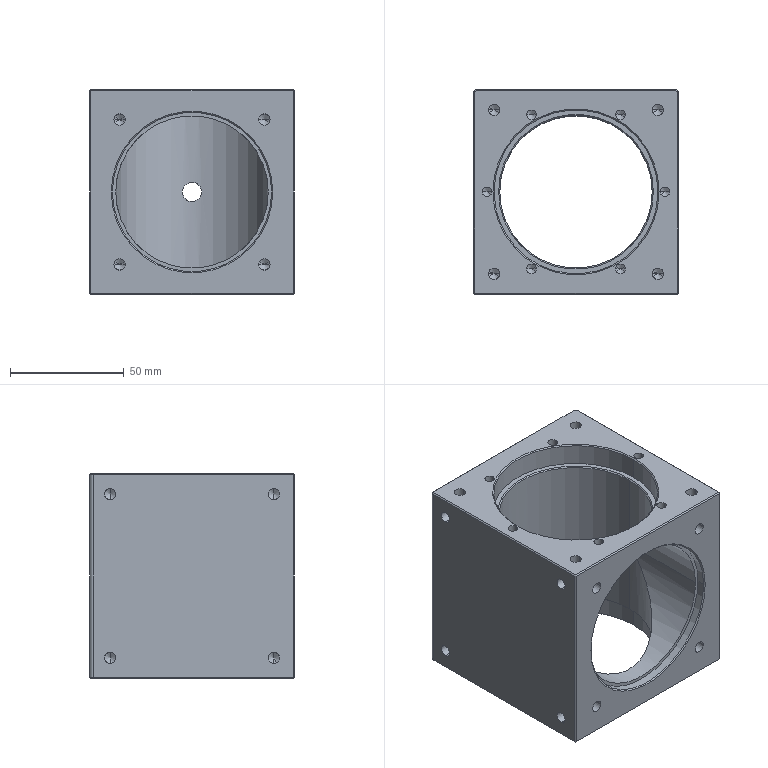NC program | NX | posted with a generic post | part box 90 x 90 x 90 mm
Whole program:
N10 G17 G21 G94 G90
(DRILLING_COPY_1_COPY_1 , TOOL : D6A45)
N12 T07 M6
N14 G54
N16 G17 G0 G90 X-31.82 Y-31.82 B0. C0. S5000 M3
N18 G43 Z30. H7
N20 G94 G81 G98 Z-1. F250. R3.
N22 Y31.82
N24 X0. Y0.
N26 X31.82 Y31.82
N28 Y-31.82
N30 G80
N32 G0 X31.82 Y-31.82 Z30.
N34 M5
(DRILLING_COPY_1_COPY_COPY_COPY_COPY , TOOL : 5.0ZT)
N36 T15 M6
N38 G54
N40 G17 G0 G90 X-31.82 Y-31.82 B0. C0. S2000 M3
N42 G43 Z30. H15
N44 G94 G83 G98 Z-18.502 F150. Q2. R3.
N46 Y31.82
N48 X31.82
N50 Y-31.82
N52 G80
N54 G0 X31.82 Y-31.82 Z30.
N56 M5
(DRILLING_COPY_1_COPY_COPY_COPY_COPY_COPY , TOOL : 9.0ZT)
N58 T09 M6
N60 G54
N62 G17 G0 G90 X0. Y0. B0. C0. S1200 M3
N64 G43 Z30. H9
N66 G94 G83 G98 Z-49.204 F150. Q2. R3.
N68 G80
N70 G0 X0. Y0. Z30.
N72 M5
(HOLE_MILLING , TOOL : D10)
N74 T10 M6
N76 G54
N78 G17 G0 G90 X0. Y0. B0. C0. S9500 M3
N80 G43 Z30. H10
N82 Z0.5
N84 G94 G3 X-1.25 Y1.25 R1.25 F2200.
N86 X-2.5 Y0. R1.25
N88 X-2.5 Y0. Z-0.5 I2.5 J0.
N90 X-2.5 Y0. Z-1.5 I2.5 J0.
N92 X-2.5 Y0. Z-2.5 I2.5 J0.
N94 X-2.5 Y0. Z-3.5 I2.5 J0.
N96 X0.096 Y-2.678 R2.68
N98 X2.986 Y-0.171 R2.819
N100 X0.343 Y3.215 R3.076
N102 X-3.459 Y0.397 R3.389
N104 X-0.596 Y-3.677 R3.567
N106 X3.915 Y-0.677 R3.881
N108 X0.902 Y4.119 R4.059
N110 X-4.348 Y1.011 R4.372
N112 X-1.261 Y-4.535 R4.55
N114 X4.754 Y-1.396 R4.863
N116 X1.669 Y4.923 R5.041
N118 X-5.129 Y1.83 R5.354
N120 X-2.126 Y-5.277 R5.532
N122 X5.468 Y-2.311 R5.845
N124 X2.627 Y5.594 R6.023
N126 X-5.768 Y2.836 R6.336
N128 X-3.172 Y-5.869 R6.514
N130 X6.024 Y-3.402 R6.827
N132 X3.755 Y6.099 R7.005
N134 X-6.233 Y4.006 R7.318
N136 X-4.374 Y-6.28 R7.496
N138 X6.391 Y-4.644 R7.809
N140 X5.025 Y6.409 R7.987
N142 X-6.496 Y5.312 R8.3
N144 X-5.705 Y-6.483 R8.478
N146 X6.544 Y-6.006 R8.791
N148 X6.408 Y6.499 R8.969
N150 X-6.532 Y6.721 R9.282
N152 X-7.13 Y-6.454 R9.46
N154 X6.459 Y-7.454 R9.773
N156 X7.867 Y6.348 R9.951
N158 X-6.323 Y8.2 R10.264
N160 X-8.613 Y-6.177 R10.442
N162 X6.122 Y-8.953 R10.755
N164 X9.365 Y5.94 R10.933
N166 X-5.854 Y9.708 R11.246
N168 X-10.116 Y-5.637 R11.424
N170 X5.519 Y-10.46 R11.737
N172 X10.862 Y5.267 R11.915
N174 X-5.117 Y11.205 R12.228
N176 X-11.598 Y-4.83 R12.406
N178 X4.647 Y-11.936 R12.719
N180 X12.317 Y4.325 R12.897
N182 X-4.11 Y12.649 R13.21
N184 X-13.015 Y-3.753 R13.388
N186 X3.506 Y-13.338 R13.701
N188 X13.686 Y3.115 R13.879
N190 X-2.836 Y13.997 R14.192
N192 X-14.325 Y-2.412 R14.37
N194 X2.102 Y-14.622 R14.683
N196 X14.927 Y1.647 R14.861
N198 X-1.306 Y15.208 R15.174
N200 X-15.487 Y-0.82 R15.352
N202 X0.45 Y-15.748 R15.665
N204 X15.999 Y-0.066 R15.843
N206 X0.464 Y16.239 R16.156
N208 X-16.46 Y1.007 R16.334
N210 X-1.432 Y-16.675 R16.647
N212 X16.863 Y-2.001 R16.825
N214 X2.452 Y17.052 R17.138
N216 X-17.205 Y3.044 R17.315
N218 X-3.519 Y-17.365 R17.629
N220 X17.481 Y-4.133 R17.806
N222 X4.629 Y17.611 R18.119
N224 X-17.688 Y5.262 R18.297
N226 X-5.779 Y-17.785 R18.61
N228 X17.821 Y-6.428 R18.788
N230 X6.963 Y17.883 R19.101
N232 X-17.877 Y7.626 R19.279
N234 X-8.176 Y-17.903 R19.592
N236 X17.853 Y-8.851 R19.77
N238 X9.414 Y17.841 R20.083
N240 X-17.746 Y10.097 R20.261
N242 X-10.671 Y-17.695 R20.574
N244 X17.554 Y-11.359 R20.752
N246 X11.941 Y17.462 R21.065
N248 X-17.274 Y12.632 R21.243
N250 X-13.218 Y-17.141 R21.556
N252 X16.905 Y-13.908 R21.734
N254 X14.496 Y16.73 R22.047
N256 X-16.445 Y15.182 R22.225
N258 X-15.77 Y-16.227 R22.538
N260 X15.893 Y-16.448 R22.716
N262 X17.032 Y15.632 R23.029
N264 X-15.25 Y17.7 R23.207
N266 X-18.277 Y-14.945 R23.52
N268 X14.514 Y-18.93 R23.697
N270 X19.497 Y14.166 R24.011
N272 X-13.687 Y20.133 R24.188
N274 X-20.687 Y-13.295 R24.501
N276 X12.769 Y-21.302 R24.679
N278 X21.84 Y12.334 R24.992
N280 X-11.761 Y22.431 R25.17
N282 X-22.949 Y-11.283 R25.483
N284 X10.665 Y-23.512 R25.661
N286 X24.008 Y10.146 R25.974
N288 X-9.484 Y24.54 R26.152
N290 X-25.01 Y-8.924 R26.465
N292 X8.219 Y-25.508 R26.643
N294 X25.95 Y7.62 R26.956
N296 X-6.874 Y26.411 R27.134
N298 X-26.821 Y-6.237 R27.447
N300 X5.453 Y-27.241 R27.625
N302 X27.617 Y4.779 R27.938
N304 X-3.958 Y27.994 R28.116
N306 X-28.332 Y-3.251 R28.429
N308 X2.396 Y-28.663 R28.607
N310 X28.962 Y1.656 R28.92
N312 X-1.003 Y29.316 R29.177
N314 X-29.5 Y0. R29.328
N316 X0. Y-29.5 R29.5
N318 X-29.5 Y0. R-29.5
N320 X-14.75 Y-14.75 R14.75
N322 X0. Y0. R14.75
N324 G0 Z30.
N326 M5
(HOLE_MILLING_COPY , TOOL : D16)
N328 T16 M6
N330 G54
N332 G17 G0 G90 X0. Y0. B0. C0. S8500 M3
N334 G43 Z30. H16
N336 Z-3.
N338 G94 G3 X-1.5 Y1.5 R1.5 F2200.
N340 X-3. Y0. R1.5
N342 X-3. Y0. Z-4. I3. J0.
N344 X-3. Y0. Z-5. I3. J0.
N346 X-3. Y0. Z-6. I3. J0.
N348 X-3. Y0. Z-7. I3. J0.
N350 X-3. Y0. Z-8. I3. J0.
N352 X-3. Y0. Z-9. I3. J0.
N354 X-3. Y0. Z-10. I3. J0.
N356 X-3. Y0. Z-11. I3. J0.
N358 X-3. Y0. Z-12. I3. J0.
N360 X-3. Y0. Z-13. I3. J0.
N362 X-3. Y0. Z-14. I3. J0.
N364 X-3. Y0. Z-15. I3. J0.
N366 X-3. Y0. Z-16. I3. J0.
N368 X-3. Y0. Z-17. I3. J0.
N370 X-3. Y0. Z-18. I3. J0.
N372 X-3. Y0. Z-19. I3. J0.
N374 X-3. Y0. Z-20. I3. J0.
N376 X-3. Y0. Z-21. I3. J0.
N378 X-3. Y0. Z-22. I3. J0.
N380 X-3. Y0. Z-23. I3. J0.
N382 X-3. Y0. Z-24. I3. J0.
N384 X0.141 Y-3.177 R3.177
N386 X3.496 Y-0.073 R3.325
N388 X0.186 Y3.738 R3.583
N390 X-3.99 Y0.167 R3.9
N392 X-0.29 Y-4.23 R4.08
N394 X4.481 Y-0.282 R4.397
N396 X0.415 Y4.718 R4.577
N398 X-4.969 Y0.417 R4.894
N400 X-0.56 Y-5.203 R5.074
N402 X5.453 Y-0.573 R5.391
N404 X0.726 Y5.684 R5.571
N406 X-5.933 Y0.749 R5.888
N408 X-0.912 Y-6.16 R6.068
N410 X6.407 Y-0.946 R6.385
N412 X1.119 Y6.63 R6.565
N414 X-6.876 Y1.163 R6.881
N416 X-1.345 Y-7.094 R7.062
N418 X7.338 Y-1.4 R7.378
N420 X1.592 Y7.551 R7.558
N422 X-7.793 Y1.656 R7.875
N424 X-1.858 Y-8.001 R8.055
N426 X8.24 Y-1.933 R8.372
N428 X2.143 Y8.443 R8.552
N430 X-8.679 Y2.228 R8.868
N432 X-2.448 Y-8.876 R9.049
N434 X9.108 Y-2.543 R9.365
N436 X2.772 Y9.3 R9.545
N438 X-9.529 Y2.877 R9.862
N440 X-3.115 Y-9.714 R10.042
N442 X9.939 Y-3.229 R10.359
N444 X3.476 Y10.117 R10.539
N446 X-10.338 Y3.6 R10.855
N448 X-3.855 Y-10.509 R11.036
N450 X10.726 Y-3.989 R11.352
N452 X4.253 Y10.89 R11.532
N454 X-11.102 Y4.395 R11.849
N456 X-4.667 Y-11.259 R12.029
N458 X11.465 Y-4.819 R12.346
N460 X5.099 Y11.614 R12.526
N462 X-11.815 Y5.26 R12.842
N464 X-5.548 Y-11.956 R13.022
N466 X12.152 Y-5.718 R13.339
N468 X6.014 Y12.285 R13.519
N470 X-12.474 Y6.192 R13.836
N472 X-6.495 Y-12.599 R14.016
N474 X12.782 Y-6.682 R14.332
N476 X6.992 Y12.898 R14.513
N478 X-13.074 Y7.188 R14.829
N480 X-7.505 Y-13.181 R15.009
N482 X13.351 Y-7.708 R15.326
N484 X8.032 Y13.449 R15.506
N486 X-13.612 Y8.244 R15.822
N488 X-8.573 Y-13.7 R16.003
N490 X13.855 Y-8.793 R16.319
N492 X9.129 Y13.934 R16.499
N494 X-14.082 Y9.356 R16.816
N496 X-9.698 Y-14.15 R16.996
N498 X14.291 Y-9.932 R17.312
N500 X10.28 Y14.349 R17.493
N502 X-14.481 Y10.521 R17.809
N504 X-10.874 Y-14.529 R17.989
N506 X14.653 Y-11.123 R18.306
N508 X11.481 Y14.691 R18.486
N510 X-14.807 Y11.736 R18.803
N512 X-12.098 Y-14.833 R18.983
N514 X14.94 Y-12.36 R19.299
N516 X12.727 Y14.956 R19.479
N518 X-15.054 Y12.994 R19.796
N520 X-13.366 Y-15.059 R19.976
N522 X15.148 Y-13.639 R20.293
N524 X14.014 Y15.141 R20.473
N526 X-15.221 Y14.293 R20.789
N528 X-14.672 Y-15.203 R20.97
N530 X15.273 Y-14.956 R21.286
N532 X15.338 Y15.243 R21.466
N534 X-15.304 Y15.628 R21.783
N536 X-16.013 Y-15.262 R21.963
N538 X15.313 Y-16.307 R22.279
N540 X16.695 Y15.26 R22.46
N542 X-15.301 Y16.993 R22.776
N544 X-17.383 Y-15.235 R22.956
N546 X15.266 Y-17.686 R23.273
N548 X18.078 Y15.189 R23.453
N550 X-15.209 Y18.384 R23.769
N552 X-18.778 Y-15.119 R23.95
N554 X15.129 Y-19.088 R24.266
N556 X19.483 Y15.027 R24.446
N558 X-15.026 Y19.796 R24.763
N560 X-20.116 Y-15.149 R25.023
N562 X14.9 Y-20.509 R25.179
N564 X20.509 Y14.9 R25.35
N566 X14.9 Y-20.509 R-25.35
N568 X17.704 Y-2.804 R12.675
N570 X0. Y0. R12.675
N572 X-1.5 Y1.5 R1.5
N574 X-3. Y0. R1.5
N576 X-3. Y0. Z-25. I3. J0.
N578 X-3. Y0. Z-26. I3. J0.
N580 X-3. Y0. Z-27. I3. J0.
N582 X-3. Y0. Z-28. I3. J0.
N584 X-3. Y0. Z-29. I3. J0.
N586 X-3. Y0. Z-30. I3. J0.
N588 X-3. Y0. Z-31. I3. J0.
N590 X-3. Y0. Z-32. I3. J0.
N592 X-3. Y0. Z-33. I3. J0.
N594 X-3. Y0. Z-34. I3. J0.
N596 X-3. Y0. Z-35. I3. J0.
N598 X-3. Y0. Z-36. I3. J0.
N600 X-3. Y0. Z-37. I3. J0.
N602 X-3. Y0. Z-38. I3. J0.
N604 X-3. Y0. Z-39. I3. J0.
N606 X-3. Y0. Z-40. I3. J0.
N608 X-3. Y0. Z-41. I3. J0.
N610 X-3. Y0. Z-42. I3. J0.
N612 X-3. Y0. Z-43. I3. J0.
N614 X-3. Y0. Z-44. I3. J0.
N616 X-3. Y0. Z-45. I3. J0.
N618 X0.141 Y-3.177 R3.177
N620 X3.496 Y-0.073 R3.325
N622 X0.186 Y3.738 R3.583
N624 X-3.99 Y0.167 R3.9
N626 X-0.29 Y-4.23 R4.08
N628 X4.481 Y-0.282 R4.397
N630 X0.415 Y4.718 R4.577
N632 X-4.969 Y0.417 R4.894
N634 X-0.56 Y-5.203 R5.074
N636 X5.453 Y-0.573 R5.391
N638 X0.726 Y5.684 R5.571
N640 X-5.933 Y0.749 R5.888
N642 X-0.912 Y-6.16 R6.068
N644 X6.407 Y-0.946 R6.385
N646 X1.119 Y6.63 R6.565
N648 X-6.876 Y1.163 R6.881
N650 X-1.345 Y-7.094 R7.062
N652 X7.338 Y-1.4 R7.378
N654 X1.592 Y7.551 R7.558
N656 X-7.793 Y1.656 R7.875
N658 X-1.858 Y-8.001 R8.055
N660 X8.24 Y-1.933 R8.372
N662 X2.143 Y8.443 R8.552
N664 X-8.679 Y2.228 R8.868
N666 X-2.448 Y-8.876 R9.049
N668 X9.108 Y-2.543 R9.365
N670 X2.772 Y9.3 R9.545
N672 X-9.529 Y2.877 R9.862
N674 X-3.115 Y-9.714 R10.042
N676 X9.939 Y-3.229 R10.359
N678 X3.476 Y10.117 R10.539
N680 X-10.338 Y3.6 R10.855
N682 X-3.855 Y-10.509 R11.036
N684 X10.726 Y-3.989 R11.352
N686 X4.253 Y10.89 R11.532
N688 X-11.102 Y4.395 R11.849
N690 X-4.667 Y-11.259 R12.029
N692 X11.465 Y-4.819 R12.346
N694 X5.099 Y11.614 R12.526
N696 X-11.815 Y5.26 R12.842
N698 X-5.548 Y-11.956 R13.022
N700 X12.152 Y-5.718 R13.339
N702 X6.014 Y12.285 R13.519
N704 X-12.474 Y6.192 R13.836
N706 X-6.495 Y-12.599 R14.016
N708 X12.782 Y-6.682 R14.332
N710 X6.992 Y12.898 R14.513
N712 X-13.074 Y7.188 R14.829
N714 X-7.505 Y-13.181 R15.009
N716 X13.351 Y-7.708 R15.326
N718 X8.032 Y13.449 R15.506
N720 X-13.612 Y8.244 R15.822
N722 X-8.573 Y-13.7 R16.003
N724 X13.855 Y-8.793 R16.319
N726 X9.129 Y13.934 R16.499
N728 X-14.082 Y9.356 R16.816
N730 X-9.698 Y-14.15 R16.996
N732 X14.291 Y-9.932 R17.312
N734 X10.28 Y14.349 R17.493
N736 X-14.481 Y10.521 R17.809
N738 X-10.874 Y-14.529 R17.989
N740 X14.653 Y-11.123 R18.306
N742 X11.481 Y14.691 R18.486
N744 X-14.807 Y11.736 R18.803
N746 X-12.098 Y-14.833 R18.983
N748 X14.94 Y-12.36 R19.299
N750 X12.727 Y14.956 R19.479
N752 X-15.054 Y12.994 R19.796
N754 X-13.366 Y-15.059 R19.976
N756 X15.148 Y-13.639 R20.293
N758 X14.014 Y15.141 R20.473
N760 X-15.221 Y14.293 R20.789
N762 X-14.672 Y-15.203 R20.97
N764 X15.273 Y-14.956 R21.286
N766 X15.338 Y15.243 R21.466
N768 X-15.304 Y15.628 R21.783
N770 X-16.013 Y-15.262 R21.963
N772 X15.313 Y-16.307 R22.279
N774 X16.695 Y15.26 R22.46
N776 X-15.301 Y16.993 R22.776
N778 X-17.383 Y-15.235 R22.956
N780 X15.266 Y-17.686 R23.273
N782 X18.078 Y15.189 R23.453
N784 X-15.209 Y18.384 R23.769
N786 X-18.778 Y-15.119 R23.95
N788 X15.129 Y-19.088 R24.266
N790 X19.483 Y15.027 R24.446
N792 X-15.026 Y19.796 R24.763
N794 X-20.116 Y-15.149 R25.023
N796 X14.9 Y-20.509 R25.179
N798 X20.509 Y14.9 R25.35
N800 X14.9 Y-20.509 R-25.35
N802 X17.704 Y-2.804 R12.675
N804 X0. Y0. R12.675
N806 G0 Z30.
N808 M5
(HOLE_MILLING_COPY_COPY , TOOL : D12JING)
N810 T12 M6
N812 G54
N814 G17 G0 G90 X-24.171 Y2.948 B0. C0. S8000 M3
N816 G43 Z30. H12
N818 Z-17.
N820 G94 G3 X-27.5 Y0. R2.97 F1000.
N822 X0. Y-27.5 R27.5
N824 X-27.5 Y0. R-27.5
N826 X-24.171 Y-2.948 R2.97
N828 G0 Y2.948 Z-31.
N830 G3 X-27.5 Y0. R2.97
N832 X0. Y-27.5 R27.5
N834 X-27.5 Y0. R-27.5
N836 X-24.171 Y-2.948 R2.97
N838 G0 Y2.948 Z-45.
N840 G3 X-27.5 Y0. R2.97
N842 X0. Y-27.5 R27.5
N844 X-27.5 Y0. R-27.5
N846 X-24.171 Y-2.948 R2.97
N848 G0 Z30.
N850 M5
(ZLEVEL_PROFILE_1_COPY_1_COPY , TOOL : D6A45)
N852 T07 M6
N854 G54
N856 G17 G0 G90 X-32.861 Y31.82 B0. C0. S9500 M3
N858 G43 Z30. H7
N860 Z1.
N862 G94 G1 Z-1.5 F1000.
N864 G3 X-31.819 Y30.778 R1.041
N866 X-32.861 Y31.82 R-1.041
N868 X-32.561 Y31.3 R0.6
N870 G1 Z-0.5
N872 G0 Z30.
N874 X-32.861 Y-31.82
N876 Z1.
N878 G1 Z-1.5
N880 G3 X-31.82 Y-32.861 R1.041
N882 X-32.861 Y-31.82 R-1.041
N884 X-32.561 Y-32.339 R0.6
N886 G1 Z-0.5
N888 G0 Z30.
N890 X-1.049 Y-32.825
N892 Z-0.5
N894 G1 Z-1.5
N896 X-0.52 Y-33.741
N898 G3 X0. Y-34.041 R0.6
N900 X34.041 Y0. R34.041
N902 X0. Y-34.041 R-34.041
N904 X0.52 Y-33.741 R0.6
N906 G1 X1.049 Y-32.825
N908 Z-0.5
N910 G0 Z30.
N912 X32.861 Y31.82
N914 Z1.
N916 G1 Z-1.5
N918 Y31.825
N920 G3 X31.815 Y32.861 R1.041
N922 X32.861 Y31.82 R-1.041
N924 X32.561 Y32.339 R0.6
N926 G1 Z-0.5
N928 G0 Z30.
N930 X32.861 Y-31.82
N932 Z1.
N934 G1 Z-1.5
N936 G3 X31.82 Y-30.778 R1.041
N938 X32.861 Y-31.82 R-1.041
N940 X32.561 Y-31.3 R0.6
N942 G1 Z-0.5
N944 G0 Z30.
N946 X45.441 Y-46.987
N948 Z-0.5
N950 G1 Z-1.5
N952 X45.02 Y-46.259
N954 G3 X44.501 Y-45.959 R0.6
N956 G1 X-44.501
N958 G2 X-45.959 Y-44.501 R1.458
N960 G1 Y44.501
N962 G2 X-44.501 Y45.959 R1.458
N964 G1 X44.501
N966 G2 X45.959 Y44.501 R1.458
N968 G1 Y-44.501
N970 G2 X44.501 Y-45.959 R1.458
N972 G3 X43.981 Y-46.259 R0.6
N974 G1 X43.462 Y-47.159
N976 Z-0.5
N978 G0 Z30.
N980 M5
N982 M2